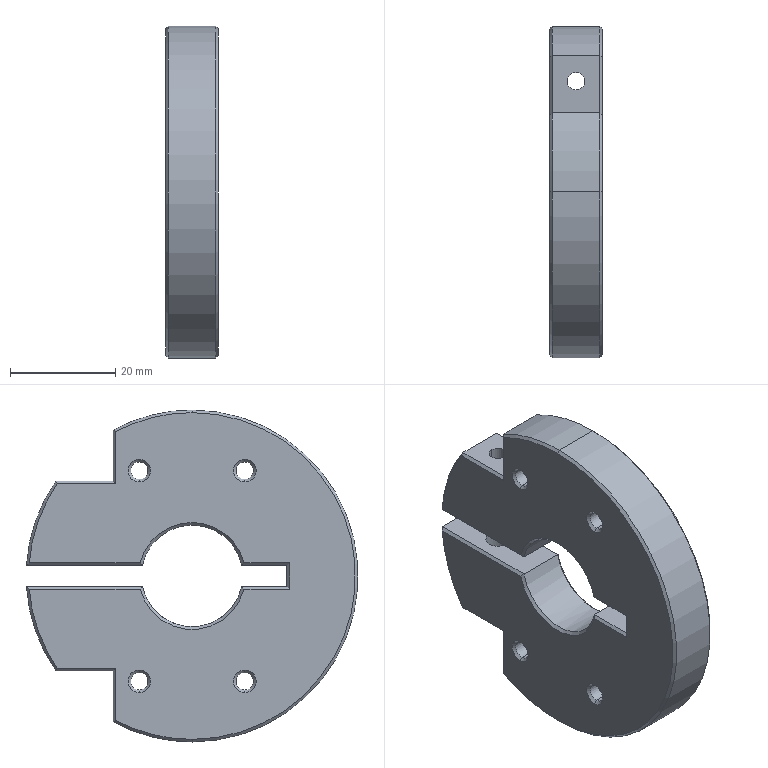Part | SolidWorks | features HoleWzd 3, Chamfer 1, Extrusion 1 | 1 solid | 84 faces | box 10 x 62.936 x 63 mm | volume 24833 mm3 | cone 32 | plane 30 | cylinder 22 | commonest cylinder face diameters 3.3 x10 63 x5 19.3 x3 4.5 x2 8 x2